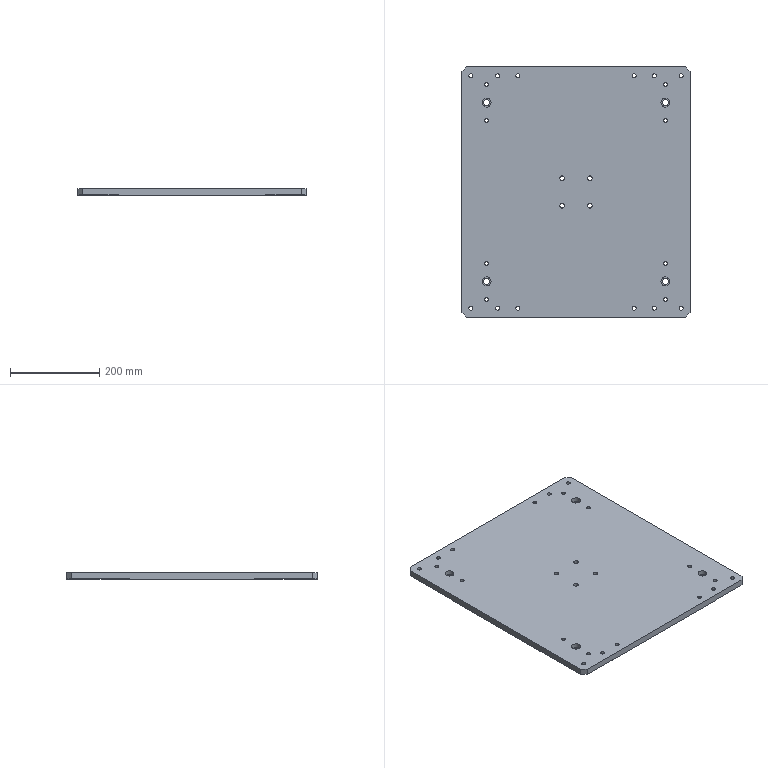Part | SolidWorks | features BaseBody 1 | 1 solid | 130 faces | box 510 x 560 x 15 mm | volume 4182002 mm3 | cylinder 92 | plane 38 | commonest cylinder face diameters 9 x24 15 x24 8.5 x16 10.2 x8 13.5 x8 20 x8